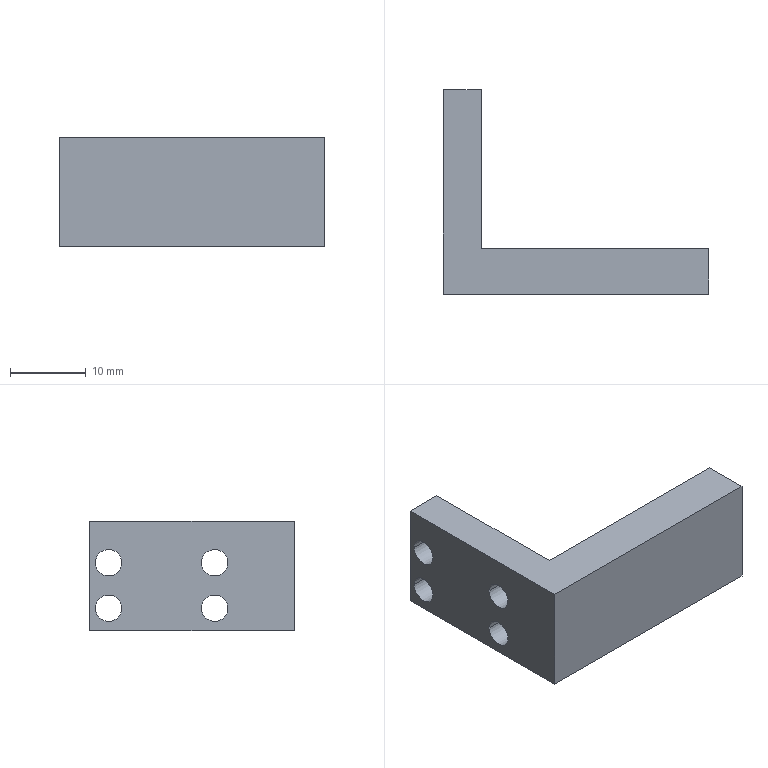Part | SolidWorks | features BaseBody 1 | 1 solid | 16 faces | box 35 x 27 x 14.5 mm | volume 4375 mm3 | cylinder 8 | plane 8 | commonest cylinder face diameters 3.5 x8
STEP:
#1=CARTESIAN_POINT('',(-24.481,84.027,9.));
#2=VERTEX_POINT('',#1);
#3=CARTESIAN_POINT('',(-24.481,87.527,9.));
#4=VERTEX_POINT('',#3);
#5=CARTESIAN_POINT('',(-24.481,85.777,9.));
#6=DIRECTION('',(1.,0.,0.));
#7=DIRECTION('',(0.,1.,0.));
#8=AXIS2_PLACEMENT_3D('',#5,#6,#7);
#9=CIRCLE('',#8,1.75);
#10=EDGE_CURVE('',#2,#4,#9,.T.);
#11=ORIENTED_EDGE('',*,*,#10,.F.);
#12=CARTESIAN_POINT('',(-19.481,84.027,9.));
#13=VERTEX_POINT('',#12);
#14=CARTESIAN_POINT('',(-66.003,84.027,9.));
#15=DIRECTION('',(1.,0.,0.));
#16=VECTOR('',#15,1000.);
#17=LINE('',#14,#16);
#18=EDGE_CURVE('',#2,#13,#17,.T.);
#19=ORIENTED_EDGE('',*,*,#18,.T.);
#20=CARTESIAN_POINT('',(-19.481,87.527,9.));
#21=VERTEX_POINT('',#20);
#22=CARTESIAN_POINT('',(-19.481,85.777,9.));
#23=DIRECTION('',(1.,0.,0.));
#24=DIRECTION('',(0.,1.,0.));
#25=AXIS2_PLACEMENT_3D('',#22,#23,#24);
#26=CIRCLE('',#25,1.75);
#27=EDGE_CURVE('',#13,#21,#26,.T.);
#28=ORIENTED_EDGE('',*,*,#27,.T.);
#29=CARTESIAN_POINT('',(-66.003,87.527,9.));
#30=DIRECTION('',(1.,0.,0.));
#31=VECTOR('',#30,1000.);
#32=LINE('',#29,#31);
#33=EDGE_CURVE('',#4,#21,#32,.T.);
#34=ORIENTED_EDGE('',*,*,#33,.F.);
#35=EDGE_LOOP('',(#11,#19,#28,#34));
#36=FACE_OUTER_BOUND('',#35,.T.);
#37=CARTESIAN_POINT('',(-66.003,85.777,9.));
#38=DIRECTION('',(1.,0.,0.));
#39=DIRECTION('',(0.,1.,0.));
#40=AXIS2_PLACEMENT_3D('',#37,#38,#39);
#41=CYLINDRICAL_SURFACE('',#40,1.75);
#42=ADVANCED_FACE('',(#36),#41,.F.);
#43=CARTESIAN_POINT('',(-24.481,84.027,3.));
#44=VERTEX_POINT('',#43);
#45=CARTESIAN_POINT('',(-24.481,87.527,3.));
#46=VERTEX_POINT('',#45);
#47=CARTESIAN_POINT('',(-24.481,85.777,3.));
#48=DIRECTION('',(1.,0.,0.));
#49=DIRECTION('',(0.,1.,0.));
#50=AXIS2_PLACEMENT_3D('',#47,#48,#49);
#51=CIRCLE('',#50,1.75);
#52=EDGE_CURVE('',#44,#46,#51,.T.);
#53=ORIENTED_EDGE('',*,*,#52,.F.);
#54=CARTESIAN_POINT('',(-19.481,84.027,3.));
#55=VERTEX_POINT('',#54);
#56=CARTESIAN_POINT('',(-66.003,84.027,3.));
#57=DIRECTION('',(1.,0.,0.));
#58=VECTOR('',#57,1000.);
#59=LINE('',#56,#58);
#60=EDGE_CURVE('',#44,#55,#59,.T.);
#61=ORIENTED_EDGE('',*,*,#60,.T.);
#62=CARTESIAN_POINT('',(-19.481,87.527,3.));
#63=VERTEX_POINT('',#62);
#64=CARTESIAN_POINT('',(-19.481,85.777,3.));
#65=DIRECTION('',(1.,0.,0.));
#66=DIRECTION('',(0.,1.,0.));
#67=AXIS2_PLACEMENT_3D('',#64,#65,#66);
#68=CIRCLE('',#67,1.75);
#69=EDGE_CURVE('',#55,#63,#68,.T.);
#70=ORIENTED_EDGE('',*,*,#69,.T.);
#71=CARTESIAN_POINT('',(-66.003,87.527,3.));
#72=DIRECTION('',(1.,0.,0.));
#73=VECTOR('',#72,1000.);
#74=LINE('',#71,#73);
#75=EDGE_CURVE('',#46,#63,#74,.T.);
#76=ORIENTED_EDGE('',*,*,#75,.F.);
#77=EDGE_LOOP('',(#53,#61,#70,#76));
#78=FACE_OUTER_BOUND('',#77,.T.);
#79=CARTESIAN_POINT('',(-66.003,85.777,3.));
#80=DIRECTION('',(1.,0.,0.));
#81=DIRECTION('',(0.,1.,0.));
#82=AXIS2_PLACEMENT_3D('',#79,#80,#81);
#83=CYLINDRICAL_SURFACE('',#82,1.75);
#84=ADVANCED_FACE('',(#78),#83,.F.);
#85=CARTESIAN_POINT('',(-24.481,70.027,9.));
#86=VERTEX_POINT('',#85);
#87=CARTESIAN_POINT('',(-24.481,73.527,9.));
#88=VERTEX_POINT('',#87);
#89=CARTESIAN_POINT('',(-24.481,71.777,9.));
#90=DIRECTION('',(1.,0.,0.));
#91=DIRECTION('',(0.,1.,0.));
#92=AXIS2_PLACEMENT_3D('',#89,#90,#91);
#93=CIRCLE('',#92,1.75);
#94=EDGE_CURVE('',#86,#88,#93,.T.);
#95=ORIENTED_EDGE('',*,*,#94,.F.);
#96=CARTESIAN_POINT('',(-19.481,70.027,9.));
#97=VERTEX_POINT('',#96);
#98=CARTESIAN_POINT('',(-66.003,70.027,9.));
#99=DIRECTION('',(1.,0.,0.));
#100=VECTOR('',#99,1000.);
#101=LINE('',#98,#100);
#102=EDGE_CURVE('',#86,#97,#101,.T.);
#103=ORIENTED_EDGE('',*,*,#102,.T.);
#104=CARTESIAN_POINT('',(-19.481,73.527,9.));
#105=VERTEX_POINT('',#104);
#106=CARTESIAN_POINT('',(-19.481,71.777,9.));
#107=DIRECTION('',(1.,0.,0.));
#108=DIRECTION('',(0.,1.,0.));
#109=AXIS2_PLACEMENT_3D('',#106,#107,#108);
#110=CIRCLE('',#109,1.75);
#111=EDGE_CURVE('',#97,#105,#110,.T.);
#112=ORIENTED_EDGE('',*,*,#111,.T.);
#113=CARTESIAN_POINT('',(-66.003,73.527,9.));
#114=DIRECTION('',(1.,0.,0.));
#115=VECTOR('',#114,1000.);
#116=LINE('',#113,#115);
#117=EDGE_CURVE('',#88,#105,#116,.T.);
#118=ORIENTED_EDGE('',*,*,#117,.F.);
#119=EDGE_LOOP('',(#95,#103,#112,#118));
#120=FACE_OUTER_BOUND('',#119,.T.);
#121=CARTESIAN_POINT('',(-66.003,71.777,9.));
#122=DIRECTION('',(1.,0.,0.));
#123=DIRECTION('',(0.,1.,0.));
#124=AXIS2_PLACEMENT_3D('',#121,#122,#123);
#125=CYLINDRICAL_SURFACE('',#124,1.75);
#126=ADVANCED_FACE('',(#120),#125,.F.);
#127=CARTESIAN_POINT('',(-24.481,70.027,3.));
#128=VERTEX_POINT('',#127);
#129=CARTESIAN_POINT('',(-24.481,73.527,3.));
#130=VERTEX_POINT('',#129);
#131=CARTESIAN_POINT('',(-24.481,71.777,3.));
#132=DIRECTION('',(1.,0.,0.));
#133=DIRECTION('',(0.,1.,0.));
#134=AXIS2_PLACEMENT_3D('',#131,#132,#133);
#135=CIRCLE('',#134,1.75);
#136=EDGE_CURVE('',#128,#130,#135,.T.);
#137=ORIENTED_EDGE('',*,*,#136,.F.);
#138=CARTESIAN_POINT('',(-19.481,70.027,3.));
#139=VERTEX_POINT('',#138);
#140=CARTESIAN_POINT('',(-66.003,70.027,3.));
#141=DIRECTION('',(1.,0.,0.));
#142=VECTOR('',#141,1000.);
#143=LINE('',#140,#142);
#144=EDGE_CURVE('',#128,#139,#143,.T.);
#145=ORIENTED_EDGE('',*,*,#144,.T.);
#146=CARTESIAN_POINT('',(-19.481,73.527,3.));
#147=VERTEX_POINT('',#146);
#148=CARTESIAN_POINT('',(-19.481,71.777,3.));
#149=DIRECTION('',(1.,0.,0.));
#150=DIRECTION('',(0.,1.,0.));
#151=AXIS2_PLACEMENT_3D('',#148,#149,#150);
#152=CIRCLE('',#151,1.75);
#153=EDGE_CURVE('',#139,#147,#152,.T.);
#154=ORIENTED_EDGE('',*,*,#153,.T.);
#155=CARTESIAN_POINT('',(-66.003,73.527,3.));
#156=DIRECTION('',(1.,0.,0.));
#157=VECTOR('',#156,1000.);
#158=LINE('',#155,#157);
#159=EDGE_CURVE('',#130,#147,#158,.T.);
#160=ORIENTED_EDGE('',*,*,#159,.F.);
#161=EDGE_LOOP('',(#137,#145,#154,#160));
#162=FACE_OUTER_BOUND('',#161,.T.);
#163=CARTESIAN_POINT('',(-66.003,71.777,3.));
#164=DIRECTION('',(1.,0.,0.));
#165=DIRECTION('',(0.,1.,0.));
#166=AXIS2_PLACEMENT_3D('',#163,#164,#165);
#167=CYLINDRICAL_SURFACE('',#166,1.75);
#168=ADVANCED_FACE('',(#162),#167,.F.);
#169=CARTESIAN_POINT('',(-24.481,61.277,0.));
#170=VERTEX_POINT('',#169);
#171=CARTESIAN_POINT('',(10.519,61.277,0.));
#172=VERTEX_POINT('',#171);
#173=CARTESIAN_POINT('',(10.519,61.277,0.));
#174=DIRECTION('',(1.,0.,0.));
#175=VECTOR('',#174,1000.);
#176=LINE('',#173,#175);
#177=EDGE_CURVE('',#170,#172,#176,.T.);
#178=ORIENTED_EDGE('',*,*,#177,.T.);
#179=CARTESIAN_POINT('',(10.519,61.277,14.5));
#180=VERTEX_POINT('',#179);
#181=CARTESIAN_POINT('',(10.519,61.277,0.));
#182=DIRECTION('',(0.,0.,1.));
#183=VECTOR('',#182,1000.);
#184=LINE('',#181,#183);
#185=EDGE_CURVE('',#172,#180,#184,.T.);
#186=ORIENTED_EDGE('',*,*,#185,.T.);
#187=CARTESIAN_POINT('',(-24.481,61.277,14.5));
#188=VERTEX_POINT('',#187);
#189=CARTESIAN_POINT('',(10.519,61.277,14.5));
#190=DIRECTION('',(-1.,0.,0.));
#191=VECTOR('',#190,1000.);
#192=LINE('',#189,#191);
#193=EDGE_CURVE('',#180,#188,#192,.T.);
#194=ORIENTED_EDGE('',*,*,#193,.T.);
#195=CARTESIAN_POINT('',(-24.481,61.277,0.));
#196=DIRECTION('',(0.,0.,-1.));
#197=VECTOR('',#196,1000.);
#198=LINE('',#195,#197);
#199=EDGE_CURVE('',#188,#170,#198,.T.);
#200=ORIENTED_EDGE('',*,*,#199,.T.);
#201=EDGE_LOOP('',(#178,#186,#194,#200));
#202=FACE_OUTER_BOUND('',#201,.T.);
#203=CARTESIAN_POINT('',(10.519,61.277,0.));
#204=DIRECTION('',(0.,-1.,0.));
#205=DIRECTION('',(0.,0.,-1.));
#206=AXIS2_PLACEMENT_3D('',#203,#204,#205);
#207=PLANE('',#206);
#208=ADVANCED_FACE('',(#202),#207,.T.);
#209=ORIENTED_EDGE('',*,*,#185,.F.);
#210=CARTESIAN_POINT('',(10.519,67.277,0.));
#211=VERTEX_POINT('',#210);
#212=CARTESIAN_POINT('',(10.519,88.277,0.));
#213=DIRECTION('',(0.,1.,0.));
#214=VECTOR('',#213,1000.);
#215=LINE('',#212,#214);
#216=EDGE_CURVE('',#172,#211,#215,.T.);
#217=ORIENTED_EDGE('',*,*,#216,.T.);
#218=CARTESIAN_POINT('',(10.519,67.277,14.5));
#219=VERTEX_POINT('',#218);
#220=CARTESIAN_POINT('',(10.519,67.277,0.));
#221=DIRECTION('',(0.,0.,1.));
#222=VECTOR('',#221,1000.);
#223=LINE('',#220,#222);
#224=EDGE_CURVE('',#211,#219,#223,.T.);
#225=ORIENTED_EDGE('',*,*,#224,.T.);
#226=CARTESIAN_POINT('',(10.519,88.277,14.5));
#227=DIRECTION('',(0.,-1.,0.));
#228=VECTOR('',#227,1000.);
#229=LINE('',#226,#228);
#230=EDGE_CURVE('',#219,#180,#229,.T.);
#231=ORIENTED_EDGE('',*,*,#230,.T.);
#232=EDGE_LOOP('',(#209,#217,#225,#231));
#233=FACE_OUTER_BOUND('',#232,.T.);
#234=CARTESIAN_POINT('',(10.519,88.277,0.));
#235=DIRECTION('',(1.,0.,0.));
#236=DIRECTION('',(0.,0.,-1.));
#237=AXIS2_PLACEMENT_3D('',#234,#235,#236);
#238=PLANE('',#237);
#239=ADVANCED_FACE('',(#233),#238,.T.);
#240=CARTESIAN_POINT('',(-19.481,67.277,0.));
#241=VERTEX_POINT('',#240);
#242=CARTESIAN_POINT('',(-6.981,67.277,0.));
#243=DIRECTION('',(-1.,0.,0.));
#244=VECTOR('',#243,1000.);
#245=LINE('',#242,#244);
#246=EDGE_CURVE('',#211,#241,#245,.T.);
#247=ORIENTED_EDGE('',*,*,#246,.F.);
#248=ORIENTED_EDGE('',*,*,#216,.F.);
#249=ORIENTED_EDGE('',*,*,#177,.F.);
#250=CARTESIAN_POINT('',(-24.481,88.277,0.));
#251=VERTEX_POINT('',#250);
#252=CARTESIAN_POINT('',(-24.481,74.777,0.));
#253=DIRECTION('',(0.,-1.,0.));
#254=VECTOR('',#253,1000.);
#255=LINE('',#252,#254);
#256=EDGE_CURVE('',#251,#170,#255,.T.);
#257=ORIENTED_EDGE('',*,*,#256,.F.);
#258=CARTESIAN_POINT('',(-19.481,88.277,0.));
#259=VERTEX_POINT('',#258);
#260=CARTESIAN_POINT('',(-6.981,88.277,0.));
#261=DIRECTION('',(-1.,0.,0.));
#262=VECTOR('',#261,1000.);
#263=LINE('',#260,#262);
#264=EDGE_CURVE('',#259,#251,#263,.T.);
#265=ORIENTED_EDGE('',*,*,#264,.F.);
#266=CARTESIAN_POINT('',(-19.481,74.777,0.));
#267=DIRECTION('',(0.,1.,0.));
#268=VECTOR('',#267,1000.);
#269=LINE('',#266,#268);
#270=EDGE_CURVE('',#241,#259,#269,.T.);
#271=ORIENTED_EDGE('',*,*,#270,.F.);
#272=EDGE_LOOP('',(#247,#248,#249,#257,#265,#271));
#273=FACE_OUTER_BOUND('',#272,.T.);
#274=CARTESIAN_POINT('',(-6.981,74.777,0.));
#275=DIRECTION('',(0.,0.,1.));
#276=DIRECTION('',(1.,0.,0.));
#277=AXIS2_PLACEMENT_3D('',#274,#275,#276);
#278=PLANE('',#277);
#279=ADVANCED_FACE('',(#273),#278,.F.);
#280=CARTESIAN_POINT('',(-24.481,85.777,9.));
#281=DIRECTION('',(1.,0.,0.));
#282=DIRECTION('',(0.,1.,0.));
#283=AXIS2_PLACEMENT_3D('',#280,#281,#282);
#284=CIRCLE('',#283,1.75);
#285=EDGE_CURVE('',#4,#2,#284,.T.);
#286=ORIENTED_EDGE('',*,*,#285,.T.);
#287=ORIENTED_EDGE('',*,*,#10,.T.);
#288=EDGE_LOOP('',(#286,#287));
#289=FACE_BOUND('',#288,.T.);
#290=CARTESIAN_POINT('',(-24.481,85.777,3.));
#291=DIRECTION('',(1.,0.,0.));
#292=DIRECTION('',(0.,1.,0.));
#293=AXIS2_PLACEMENT_3D('',#290,#291,#292);
#294=CIRCLE('',#293,1.75);
#295=EDGE_CURVE('',#46,#44,#294,.T.);
#296=ORIENTED_EDGE('',*,*,#295,.T.);
#297=ORIENTED_EDGE('',*,*,#52,.T.);
#298=EDGE_LOOP('',(#296,#297));
#299=FACE_BOUND('',#298,.T.);
#300=CARTESIAN_POINT('',(-24.481,71.777,9.));
#301=DIRECTION('',(1.,0.,0.));
#302=DIRECTION('',(0.,1.,0.));
#303=AXIS2_PLACEMENT_3D('',#300,#301,#302);
#304=CIRCLE('',#303,1.75);
#305=EDGE_CURVE('',#88,#86,#304,.T.);
#306=ORIENTED_EDGE('',*,*,#305,.T.);
#307=ORIENTED_EDGE('',*,*,#94,.T.);
#308=EDGE_LOOP('',(#306,#307));
#309=FACE_BOUND('',#308,.T.);
#310=CARTESIAN_POINT('',(-24.481,71.777,3.));
#311=DIRECTION('',(1.,0.,0.));
#312=DIRECTION('',(0.,1.,0.));
#313=AXIS2_PLACEMENT_3D('',#310,#311,#312);
#314=CIRCLE('',#313,1.75);
#315=EDGE_CURVE('',#130,#128,#314,.T.);
#316=ORIENTED_EDGE('',*,*,#315,.T.);
#317=ORIENTED_EDGE('',*,*,#136,.T.);
#318=EDGE_LOOP('',(#316,#317));
#319=FACE_BOUND('',#318,.T.);
#320=ORIENTED_EDGE('',*,*,#256,.T.);
#321=ORIENTED_EDGE('',*,*,#199,.F.);
#322=CARTESIAN_POINT('',(-24.481,88.277,14.5));
#323=VERTEX_POINT('',#322);
#324=CARTESIAN_POINT('',(-24.481,61.277,14.5));
#325=DIRECTION('',(0.,1.,0.));
#326=VECTOR('',#325,1000.);
#327=LINE('',#324,#326);
#328=EDGE_CURVE('',#188,#323,#327,.T.);
#329=ORIENTED_EDGE('',*,*,#328,.T.);
#330=CARTESIAN_POINT('',(-24.481,88.277,0.));
#331=DIRECTION('',(0.,0.,-1.));
#332=VECTOR('',#331,1000.);
#333=LINE('',#330,#332);
#334=EDGE_CURVE('',#323,#251,#333,.T.);
#335=ORIENTED_EDGE('',*,*,#334,.T.);
#336=EDGE_LOOP('',(#320,#321,#329,#335));
#337=FACE_OUTER_BOUND('',#336,.T.);
#338=CARTESIAN_POINT('',(-24.481,61.277,0.));
#339=DIRECTION('',(-1.,0.,0.));
#340=DIRECTION('',(0.,0.,1.));
#341=AXIS2_PLACEMENT_3D('',#338,#339,#340);
#342=PLANE('',#341);
#343=ADVANCED_FACE('',(#289,#299,#309,#319,#337),#342,.T.);
#344=ORIENTED_EDGE('',*,*,#193,.F.);
#345=ORIENTED_EDGE('',*,*,#230,.F.);
#346=CARTESIAN_POINT('',(-19.481,67.277,14.5));
#347=VERTEX_POINT('',#346);
#348=CARTESIAN_POINT('',(-6.981,67.277,14.5));
#349=DIRECTION('',(-1.,0.,0.));
#350=VECTOR('',#349,1000.);
#351=LINE('',#348,#350);
#352=EDGE_CURVE('',#219,#347,#351,.T.);
#353=ORIENTED_EDGE('',*,*,#352,.T.);
#354=CARTESIAN_POINT('',(-19.481,88.277,14.5));
#355=VERTEX_POINT('',#354);
#356=CARTESIAN_POINT('',(-19.481,74.777,14.5));
#357=DIRECTION('',(0.,1.,0.));
#358=VECTOR('',#357,1000.);
#359=LINE('',#356,#358);
#360=EDGE_CURVE('',#347,#355,#359,.T.);
#361=ORIENTED_EDGE('',*,*,#360,.T.);
#362=CARTESIAN_POINT('',(-6.981,88.277,14.5));
#363=DIRECTION('',(-1.,0.,0.));
#364=VECTOR('',#363,1000.);
#365=LINE('',#362,#364);
#366=EDGE_CURVE('',#355,#323,#365,.T.);
#367=ORIENTED_EDGE('',*,*,#366,.T.);
#368=ORIENTED_EDGE('',*,*,#328,.F.);
#369=EDGE_LOOP('',(#344,#345,#353,#361,#367,#368));
#370=FACE_OUTER_BOUND('',#369,.T.);
#371=CARTESIAN_POINT('',(-6.981,74.777,14.5));
#372=DIRECTION('',(0.,0.,1.));
#373=DIRECTION('',(1.,0.,0.));
#374=AXIS2_PLACEMENT_3D('',#371,#372,#373);
#375=PLANE('',#374);
#376=ADVANCED_FACE('',(#370),#375,.T.);
#377=CARTESIAN_POINT('',(-19.481,67.277,14.5));
#378=DIRECTION('',(0.,0.,-1.));
#379=VECTOR('',#378,1000.);
#380=LINE('',#377,#379);
#381=EDGE_CURVE('',#347,#241,#380,.T.);
#382=ORIENTED_EDGE('',*,*,#381,.F.);
#383=ORIENTED_EDGE('',*,*,#352,.F.);
#384=ORIENTED_EDGE('',*,*,#224,.F.);
#385=ORIENTED_EDGE('',*,*,#246,.T.);
#386=EDGE_LOOP('',(#382,#383,#384,#385));
#387=FACE_OUTER_BOUND('',#386,.T.);
#388=CARTESIAN_POINT('',(-19.481,67.277,14.5));
#389=DIRECTION('',(0.,-1.,0.));
#390=DIRECTION('',(0.,0.,-1.));
#391=AXIS2_PLACEMENT_3D('',#388,#389,#390);
#392=PLANE('',#391);
#393=ADVANCED_FACE('',(#387),#392,.F.);
#394=CARTESIAN_POINT('',(-19.481,85.777,9.));
#395=DIRECTION('',(1.,0.,0.));
#396=DIRECTION('',(0.,1.,0.));
#397=AXIS2_PLACEMENT_3D('',#394,#395,#396);
#398=CIRCLE('',#397,1.75);
#399=EDGE_CURVE('',#21,#13,#398,.T.);
#400=ORIENTED_EDGE('',*,*,#399,.F.);
#401=ORIENTED_EDGE('',*,*,#27,.F.);
#402=EDGE_LOOP('',(#400,#401));
#403=FACE_BOUND('',#402,.T.);
#404=CARTESIAN_POINT('',(-19.481,85.777,3.));
#405=DIRECTION('',(1.,0.,0.));
#406=DIRECTION('',(0.,1.,0.));
#407=AXIS2_PLACEMENT_3D('',#404,#405,#406);
#408=CIRCLE('',#407,1.75);
#409=EDGE_CURVE('',#63,#55,#408,.T.);
#410=ORIENTED_EDGE('',*,*,#409,.F.);
#411=ORIENTED_EDGE('',*,*,#69,.F.);
#412=EDGE_LOOP('',(#410,#411));
#413=FACE_BOUND('',#412,.T.);
#414=CARTESIAN_POINT('',(-19.481,71.777,9.));
#415=DIRECTION('',(1.,0.,0.));
#416=DIRECTION('',(0.,1.,0.));
#417=AXIS2_PLACEMENT_3D('',#414,#415,#416);
#418=CIRCLE('',#417,1.75);
#419=EDGE_CURVE('',#105,#97,#418,.T.);
#420=ORIENTED_EDGE('',*,*,#419,.F.);
#421=ORIENTED_EDGE('',*,*,#111,.F.);
#422=EDGE_LOOP('',(#420,#421));
#423=FACE_BOUND('',#422,.T.);
#424=CARTESIAN_POINT('',(-19.481,71.777,3.));
#425=DIRECTION('',(1.,0.,0.));
#426=DIRECTION('',(0.,1.,0.));
#427=AXIS2_PLACEMENT_3D('',#424,#425,#426);
#428=CIRCLE('',#427,1.75);
#429=EDGE_CURVE('',#147,#139,#428,.T.);
#430=ORIENTED_EDGE('',*,*,#429,.F.);
#431=ORIENTED_EDGE('',*,*,#153,.F.);
#432=EDGE_LOOP('',(#430,#431));
#433=FACE_BOUND('',#432,.T.);
#434=CARTESIAN_POINT('',(-19.481,88.277,14.5));
#435=DIRECTION('',(0.,0.,-1.));
#436=VECTOR('',#435,1000.);
#437=LINE('',#434,#436);
#438=EDGE_CURVE('',#355,#259,#437,.T.);
#439=ORIENTED_EDGE('',*,*,#438,.F.);
#440=ORIENTED_EDGE('',*,*,#360,.F.);
#441=ORIENTED_EDGE('',*,*,#381,.T.);
#442=ORIENTED_EDGE('',*,*,#270,.T.);
#443=EDGE_LOOP('',(#439,#440,#441,#442));
#444=FACE_OUTER_BOUND('',#443,.T.);
#445=CARTESIAN_POINT('',(-19.481,88.277,14.5));
#446=DIRECTION('',(-1.,0.,0.));
#447=DIRECTION('',(0.,0.,1.));
#448=AXIS2_PLACEMENT_3D('',#445,#446,#447);
#449=PLANE('',#448);
#450=ADVANCED_FACE('',(#403,#413,#423,#433,#444),#449,.F.);
#451=ORIENTED_EDGE('',*,*,#334,.F.);
#452=ORIENTED_EDGE('',*,*,#366,.F.);
#453=ORIENTED_EDGE('',*,*,#438,.T.);
#454=ORIENTED_EDGE('',*,*,#264,.T.);
#455=EDGE_LOOP('',(#451,#452,#453,#454));
#456=FACE_OUTER_BOUND('',#455,.T.);
#457=CARTESIAN_POINT('',(-24.481,88.277,0.));
#458=DIRECTION('',(0.,1.,0.));
#459=DIRECTION('',(0.,0.,1.));
#460=AXIS2_PLACEMENT_3D('',#457,#458,#459);
#461=PLANE('',#460);
#462=ADVANCED_FACE('',(#456),#461,.T.);
#463=ORIENTED_EDGE('',*,*,#18,.F.);
#464=ORIENTED_EDGE('',*,*,#285,.F.);
#465=ORIENTED_EDGE('',*,*,#33,.T.);
#466=ORIENTED_EDGE('',*,*,#399,.T.);
#467=EDGE_LOOP('',(#463,#464,#465,#466));
#468=FACE_OUTER_BOUND('',#467,.T.);
#469=CARTESIAN_POINT('',(-66.003,85.777,9.));
#470=DIRECTION('',(1.,0.,0.));
#471=DIRECTION('',(0.,1.,0.));
#472=AXIS2_PLACEMENT_3D('',#469,#470,#471);
#473=CYLINDRICAL_SURFACE('',#472,1.75);
#474=ADVANCED_FACE('',(#468),#473,.F.);
#475=ORIENTED_EDGE('',*,*,#60,.F.);
#476=ORIENTED_EDGE('',*,*,#295,.F.);
#477=ORIENTED_EDGE('',*,*,#75,.T.);
#478=ORIENTED_EDGE('',*,*,#409,.T.);
#479=EDGE_LOOP('',(#475,#476,#477,#478));
#480=FACE_OUTER_BOUND('',#479,.T.);
#481=CARTESIAN_POINT('',(-66.003,85.777,3.));
#482=DIRECTION('',(1.,0.,0.));
#483=DIRECTION('',(0.,1.,0.));
#484=AXIS2_PLACEMENT_3D('',#481,#482,#483);
#485=CYLINDRICAL_SURFACE('',#484,1.75);
#486=ADVANCED_FACE('',(#480),#485,.F.);
#487=ORIENTED_EDGE('',*,*,#102,.F.);
#488=ORIENTED_EDGE('',*,*,#305,.F.);
#489=ORIENTED_EDGE('',*,*,#117,.T.);
#490=ORIENTED_EDGE('',*,*,#419,.T.);
#491=EDGE_LOOP('',(#487,#488,#489,#490));
#492=FACE_OUTER_BOUND('',#491,.T.);
#493=CARTESIAN_POINT('',(-66.003,71.777,9.));
#494=DIRECTION('',(1.,0.,0.));
#495=DIRECTION('',(0.,1.,0.));
#496=AXIS2_PLACEMENT_3D('',#493,#494,#495);
#497=CYLINDRICAL_SURFACE('',#496,1.75);
#498=ADVANCED_FACE('',(#492),#497,.F.);
#499=ORIENTED_EDGE('',*,*,#144,.F.);
#500=ORIENTED_EDGE('',*,*,#315,.F.);
#501=ORIENTED_EDGE('',*,*,#159,.T.);
#502=ORIENTED_EDGE('',*,*,#429,.T.);
#503=EDGE_LOOP('',(#499,#500,#501,#502));
#504=FACE_OUTER_BOUND('',#503,.T.);
#505=CARTESIAN_POINT('',(-66.003,71.777,3.));
#506=DIRECTION('',(1.,0.,0.));
#507=DIRECTION('',(0.,1.,0.));
#508=AXIS2_PLACEMENT_3D('',#505,#506,#507);
#509=CYLINDRICAL_SURFACE('',#508,1.75);
#510=ADVANCED_FACE('',(#504),#509,.F.);
#511=CLOSED_SHELL('',(#42,#84,#126,#168,#208,#239,#279,#343,#376,#393,#450,#462,#474,#486,#498,#510));
#512=MANIFOLD_SOLID_BREP('',#511);
#513=CARTESIAN_POINT('',(0.,0.,0.));
#514=DIRECTION('',(0.,0.,1.));
#515=DIRECTION('',(1.,0.,0.));
#516=AXIS2_PLACEMENT_3D('',#513,#514,#515);
#517=(LENGTH_UNIT()NAMED_UNIT(*)SI_UNIT(.MILLI.,.METRE.));
#518=UNCERTAINTY_MEASURE_WITH_UNIT(LENGTH_MEASURE(0.00001),#517,'','');
#519=(NAMED_UNIT(*)PLANE_ANGLE_UNIT()SI_UNIT($,.RADIAN.));
#520=(NAMED_UNIT(*)SI_UNIT($,.STERADIAN.)SOLID_ANGLE_UNIT());
#521=(GEOMETRIC_REPRESENTATION_CONTEXT(3)GLOBAL_UNCERTAINTY_ASSIGNED_CONTEXT((#518))GLOBAL_UNIT_ASSIGNED_CONTEXT((#517,#519,#520))REPRESENTATION_CONTEXT('',''));
#522=ADVANCED_BREP_SHAPE_REPRESENTATION('',(#512,#516),#521);